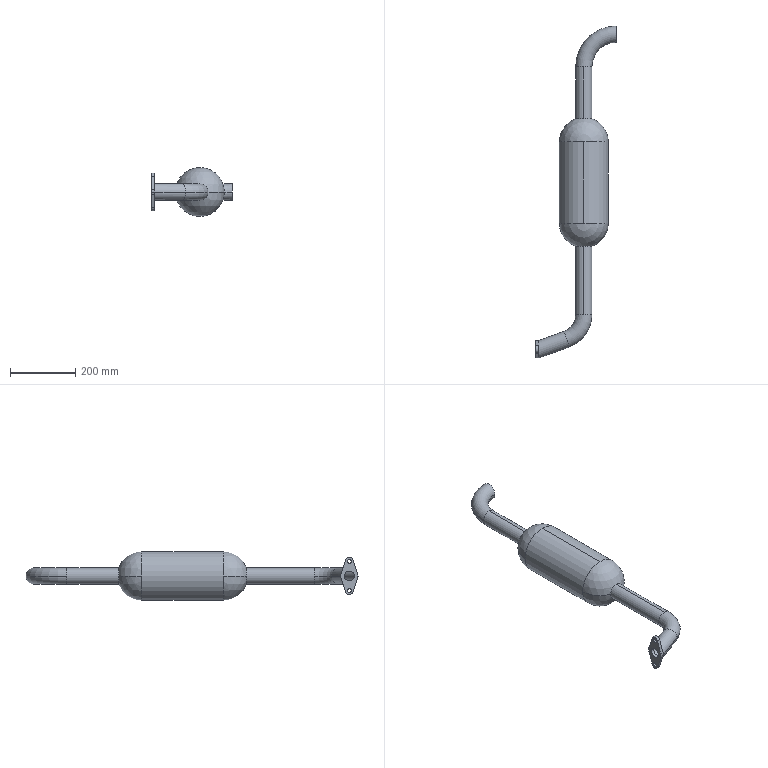Part | SolidWorks | 1 solid | 52 faces | box 248.057 x 1018 x 150 mm | volume 2628075 mm3 | cylinder 23 | torus 8 | sphere 8 | plane 8 | spline 5 | commonest cylinder face diameters 30 x6 50 x6 12 x4 25 x3 130 x2 150 x2